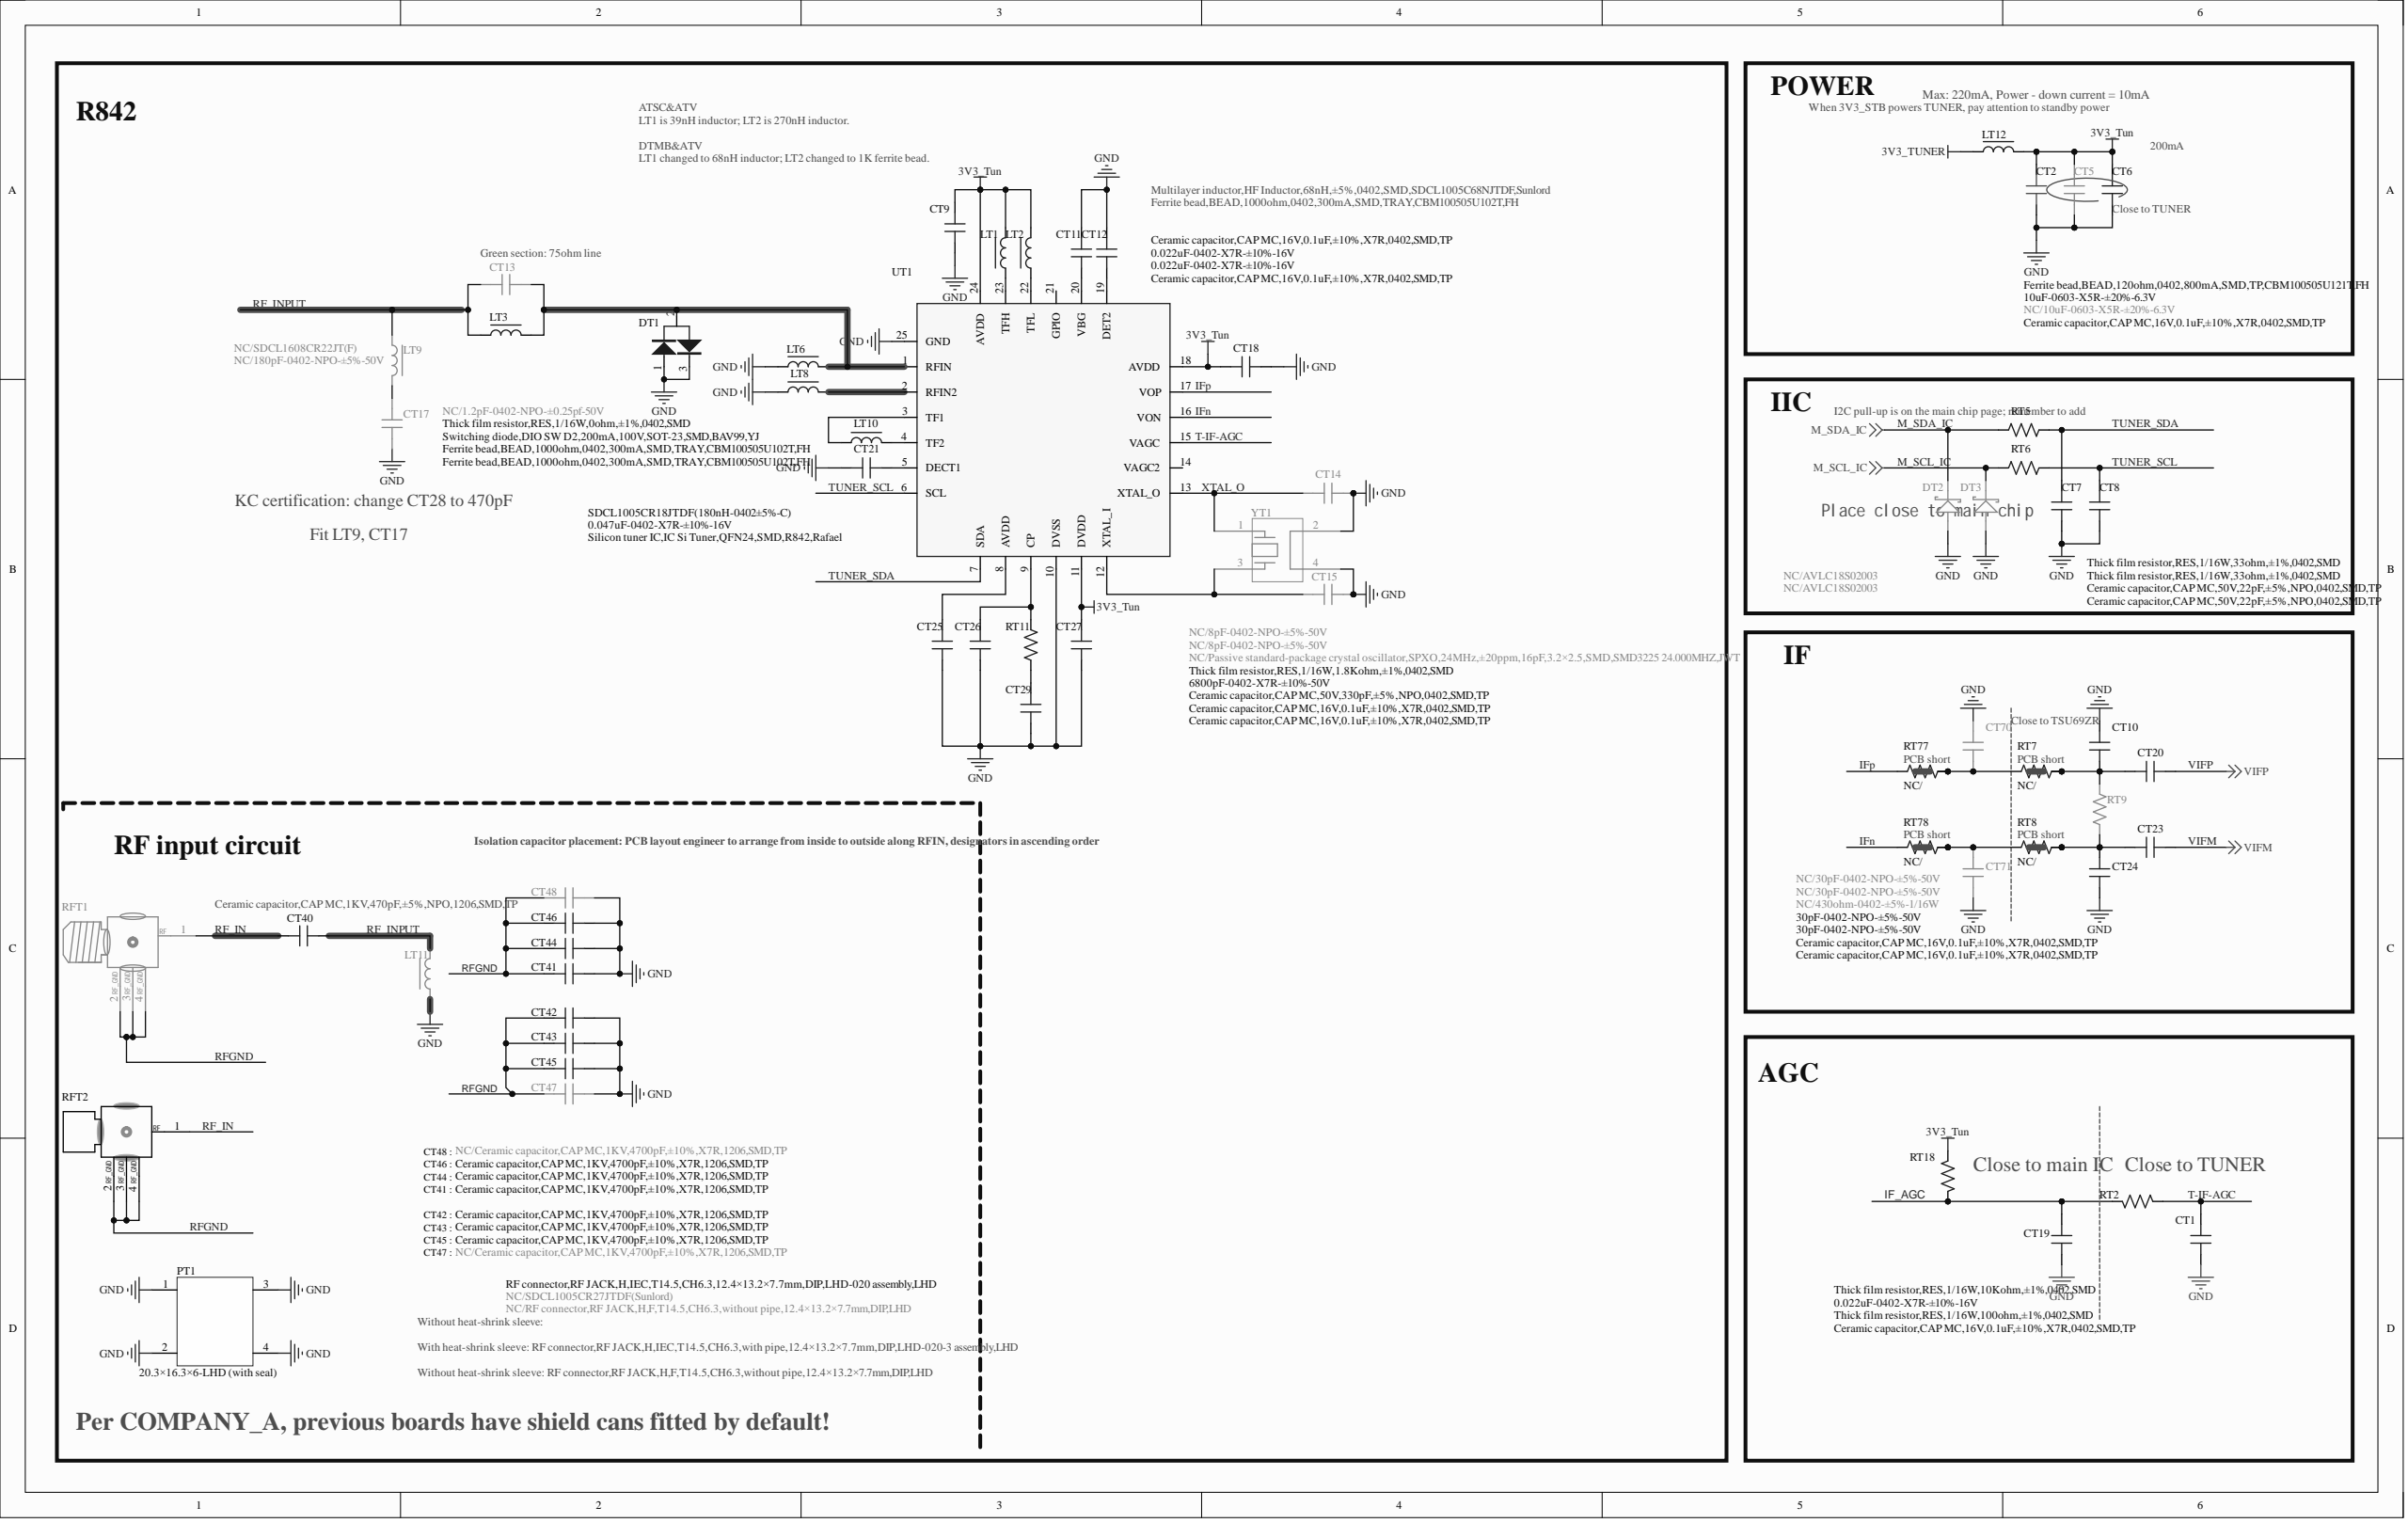Circuit board | Altium Designer | 719 parts | 352 nets | one sheet of the schematic
Parts on this sheet (reference | value | footprint):
CT1 | Ceramic capacitor,CAP MC,16V,0.1uF,±10%,X7R,0402,SMD,TP | C0402
CT2 | 10uF-0603-X5R-±20%-6.3V | C0603
CT5 | NC/10uF-0603-X5R-±20%-6.3V | C0603
CT6 | Ceramic capacitor,CAP MC,16V,0.1uF,±10%,X7R,0402,SMD,TP | C0402
CT7 | Ceramic capacitor,CAP MC,50V,22pF,±5%,NPO,0402,SMD,TP | C0402
CT8 | Ceramic capacitor,CAP MC,50V,22pF,±5%,NPO,0402,SMD,TP | C0402
CT9 | Ceramic capacitor,CAP MC,16V,0.1uF,±10%,X7R,0402,SMD,TP | C0402
CT10 | 30pF-0402-NPO-±5%-50V | C0402
CT11 | 0.022uF-0402-X7R-±10%-16V | C0402
CT12 | 0.022uF-0402-X7R-±10%-16V | C0402
CT13 | NC/1.2pF-0402-NPO-±0.25pf-50V | C0402
CT14 | NC/8pF-0402-NPO-±5%-50V | C0402
CT15 | NC/8pF-0402-NPO-±5%-50V | C0402
CT17 | NC/180pF-0402-NPO-±5%-50V | C0402
CT18 | Ceramic capacitor,CAP MC,16V,0.1uF,±10%,X7R,0402,SMD,TP | C0402
CT19 | 0.022uF-0402-X7R-±10%-16V | C0402
CT20 | Ceramic capacitor,CAP MC,16V,0.1uF,±10%,X7R,0402,SMD,TP | C0402
CT21 | 0.047uF-0402-X7R-±10%-16V | C0402
CT23 | Ceramic capacitor,CAP MC,16V,0.1uF,±10%,X7R,0402,SMD,TP | C0402
CT24 | 30pF-0402-NPO-±5%-50V | C0402
CT25 | Ceramic capacitor,CAP MC,16V,0.1uF,±10%,X7R,0402,SMD,TP | C0402
CT26 | Ceramic capacitor,CAP MC,50V,330pF,±5%,NPO,0402,SMD,TP | C0402
CT27 | Ceramic capacitor,CAP MC,16V,0.1uF,±10%,X7R,0402,SMD,TP | C0402
CT29 | 6800pF-0402-X7R-±10%-50V | C0402
CT40 | Ceramic capacitor,CAP MC,1KV,470pF,±5%,NPO,1206,SMD,TP | C1206
CT41 | Ceramic capacitor,CAP MC,1KV,4700pF,±10%,X7R,1206,SMD,TP | C1206
CT42 | Ceramic capacitor,CAP MC,1KV,4700pF,±10%,X7R,1206,SMD,TP | C1206
CT43 | Ceramic capacitor,CAP MC,1KV,4700pF,±10%,X7R,1206,SMD,TP | C1206
CT44 | Ceramic capacitor,CAP MC,1KV,4700pF,±10%,X7R,1206,SMD,TP | C1206
CT45 | Ceramic capacitor,CAP MC,1KV,4700pF,±10%,X7R,1206,SMD,TP | C1206
CT46 | Ceramic capacitor,CAP MC,1KV,4700pF,±10%,X7R,1206,SMD,TP | C1206
CT47 | NC/Ceramic capacitor,CAP MC,1KV,4700pF,±10%,X7R,1206,SMD,TP | C1206
CT48 | NC/Ceramic capacitor,CAP MC,1KV,4700pF,±10%,X7R,1206,SMD,TP | C1206
CT70 | NC/30pF-0402-NPO-±5%-50V | C0402
CT71 | NC/30pF-0402-NPO-±5%-50V | C0402
DT1 | Switching diode,DIO SW D2,200mA,100V,SOT-23,SMD,BAV99,YJ | SO-23
DT2 | NC/AVLC18S02003 | DIODE-S0402
DT3 | NC/AVLC18S02003 | DIODE-S0402
LT1 | Multilayer inductor,HF Inductor,68nH,±5%,0402,SMD,SDCL1005C68NJTDF,Sunlord | L0402
LT2 | Ferrite bead,BEAD,1000ohm,0402,300mA,SMD,TRAY,CBM100505U102T,FH | L0402
LT3 | Thick film resistor,RES,1/16W,0ohm,±1%,0402,SMD | L0402
LT6 | Ferrite bead,BEAD,1000ohm,0402,300mA,SMD,TRAY,CBM100505U102T,FH | L0402
LT8 | Ferrite bead,BEAD,1000ohm,0402,300mA,SMD,TRAY,CBM100505U102T,FH | L0402
LT9 | NC/SDCL1608CR22JT(F) | L0603
LT10 | SDCL1005CR18JTDF(180nH-0402±5%-C) | L0402
LT11 | NC/SDCL1005CR27JTDF(Sunlord) | L0402
LT12 | Ferrite bead,BEAD,120ohm,0402,800mA,SMD,TP,CBM100505U121T,FH | L0402
PT1 | 20.3×16.3×6-LHD (with seal) | SHIELD(16*20*6)
RFT1 | NC/RF connector,RF JACK,H,F,T14.5,CH6.3,without pipe,12.4×13.2×7.7mm,DIP,LHD | T-13.2×12.4×7.7-F14.5
RFT2 | RF connector,RF JACK,H,IEC,T14.5,CH6.3,12.4×13.2×7.7mm,DIP,LHD-020 assembly,LHD | ANT-IEC14.5-H-4
RT2 | Thick film resistor,RES,1/16W,100ohm,±1%,0402,SMD | R0402
RT5 | Thick film resistor,RES,1/16W,33ohm,±1%,0402,SMD | R0402
RT6 | Thick film resistor,RES,1/16W,33ohm,±1%,0402,SMD | R0402
RT7 | NC/ | R0402SC
RT8 | NC/ | R0402SC
RT9 | NC/430ohm-0402-±5%-1/16W | R0402
RT11 | Thick film resistor,RES,1/16W,1.8Kohm,±1%,0402,SMD | R0402
RT18 | Thick film resistor,RES,1/16W,10Kohm,±1%,0402,SMD | R0402
RT77 | NC/ | R0402SC
RT78 | NC/ | R0402SC
UT1 | Silicon tuner IC,IC Si Tuner,QFN24,SMD,R842,Rafael | QFN24/0.5-3
YT1 | NC/Passive standard-package crystal oscillator,SPXO,24MHz,±20ppm,16pF,3.2×2.5,SMD,SMD3225 24.000MHZ,JWT | XTAL-S-10
Nets of these parts (net: part-pin ...):
XTAL_O: CT14-2 YT1-1 UT1-13
VIFP: CT20-2
VIFM: CT23-2
TUNER_SDA: CT7-2 RT5-1 UT1-7
TUNER_SCL: CT8-2 RT6-1 UT1-6
T-IF-AGC: CT1-2 RT2-1 UT1-15
RFGND: CT41-2 CT42-2 CT43-2 CT44-2 CT45-2 CT46-2 CT47-2 CT48-2 RFT1-2 RFT1-3 RFT1-4 RFT2-2 RFT2-3 RFT2-4
RF_INPUT: CT13-1 CT40-2 LT3-1 LT9-1 LT11-1
RF_IN: CT40-1 RFT1-1 RFT2-1
NetLT10_2: LT10-2 UT1-3
NetLT10_1: LT10-1 UT1-4
NetLT8_1: LT8-1 UT1-2
NetLT2_1: LT2-1 UT1-22
NetLT1_2: LT1-2 UT1-23
NetCT71_2: CT71-2 RT8-1 RT78-2 RT78-3
NetCT70_1: CT70-1 RT7-1 RT77-2 RT77-3
NetCT29_2: CT29-2 RT11-1
NetCT26_2: CT26-2 RT11-2 UT1-9
NetCT25_1: CT25-1 UT1-8
NetCT23_1: CT23-1 CT24-2 RT8-2 RT8-3 RT9-2
NetCT21_1: CT21-1 UT1-5
NetCT17_1: CT17-1 LT9-2
NetCT15_2: CT15-2 YT1-3 UT1-12
NetCT13_2: CT13-2 DT1-2 LT3-2 LT6-1 UT1-1
NetCT12_1: CT12-1 UT1-19
NetCT11_2: CT11-2 UT1-20
NetCT10_1: CT10-1 CT20-1 RT7-2 RT7-3 RT9-1
M_SDA_IC: DT2-K RT5-2
M_SCL_IC: DT3-K RT6-2
IFp: RT77-1 UT1-17
IFn: RT78-1 UT1-16
IF_AGC: CT19-2 RT2-2 RT18-2
GND: CT1-1 CT2-1 CT5-1 CT6-2 CT7-1 CT8-1 CT9-2 CT10-2 CT11-1 CT12-2 CT14-1 CT15-1 CT17-2 CT18-1 CT19-1 CT21-2 CT24-1 CT25-2 CT26-1 CT27-2 CT29-1 CT41-1 CT42-1 CT43-1 CT44-1 CT45-1 CT46-1 CT47-1 CT48-1 CT70-2 CT71-1 DT1-1 DT1-3 DT2-A DT3-A LT6-2 LT8-2 LT11-2 PT1-1 PT1-2 PT1-3 PT1-4 YT1-2 YT1-4 UT1-10 UT1-25
3V3_TUNER: LT12-1
3V3_Tun: CT2-2 CT5-2 CT6-1 CT9-1 CT18-2 CT27-1 LT1-1 LT2-2 LT12-2 RT18-1 UT1-11 UT1-18 UT1-24